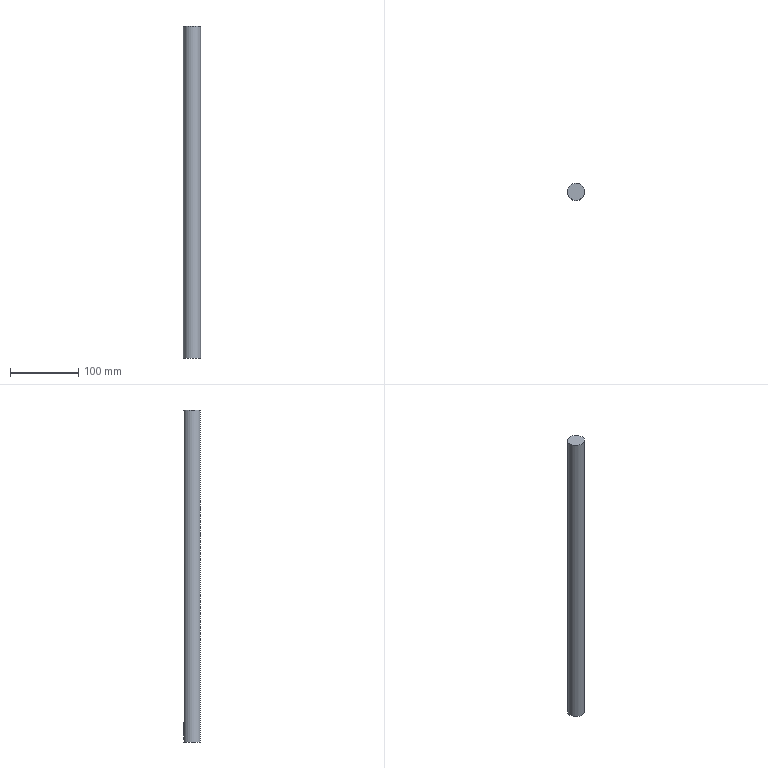CAM job | NX | 3+2 milling | part box 25 x 25 x 487 mm | stock box 25 x 25 x 487 mm
Tools:
number,name,description,diameter,corner_radius,flute_length,length,flutes
6,D6,Milling Tool-5 Parameters,6.0,0.0,50.0,75.0,2
7,D6A45,Milling Tool-5 Parameters,6.0,0.0,50.0,75.0,2
Operations:
program,operation,operation_type,tool,method,geometry_group,spindle_rpm,surface_speed,feed_per_tooth,feed_cut,feed_plunge,cut_length_mm,path_length_mm,cut_time_min,machine_time_min
1,ZLEVEL_PROFILE,ZLevelMilling,D6,METHOD,A,3800.0,71.0,0.2171,1650.0,1000.0,1816.599,1958.999,1.109,1.123
1,PROFILE_3D,PlanarMilling,D6A45,METHOD,A,7000.0,131.0,0.0893,1250.0,100.0,55.726,198.037,0.0446,0.0588
1,CUTTERCOMP6,ZLevelMilling,D6,METHOD,A,4800.0,90.0,0.1042,1000.0,1000.0,45.056,191.856,0.0451,0.0597